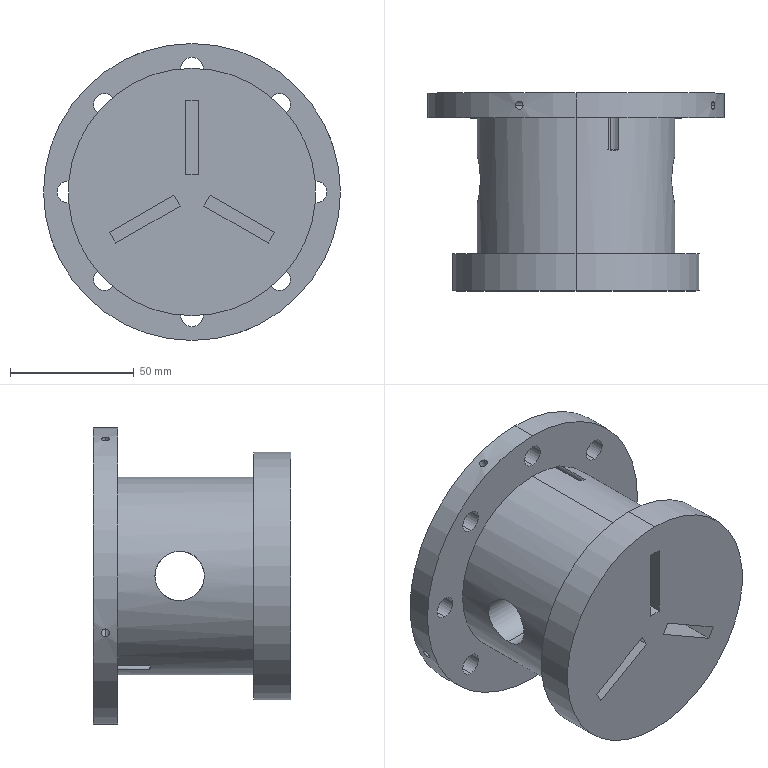Part | SolidWorks | features ICE 6, CirPattern 3, 3DProfileFeature 2, HoleWzd 2, Revolution 1 | 1 solid | 76 faces | box 120 x 80 x 120 mm | volume 422687 mm3 | cylinder 40 | plane 20 | cone 16 | commonest cylinder face diameters 9 x20 3.3 x8 20 x4 36 x2 80 x2 100 x2